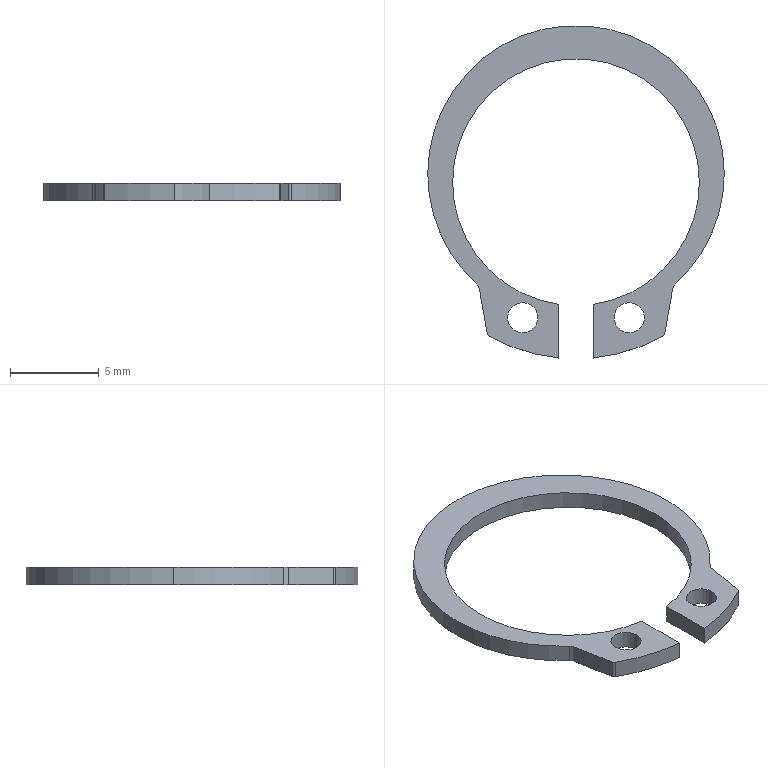Part | STEP file | 001-003-Shaft retaining ring 15-1 | 1 solid | 22 faces | box 16.7 x 18.72 x 1 mm | volume 79.464 mm3 | cylinder 16 | plane 6 | commonest cylinder face diameters 1.7 x4 13.9 x3 16.7 x3 0.4 x2 1 x2 19.9 x2